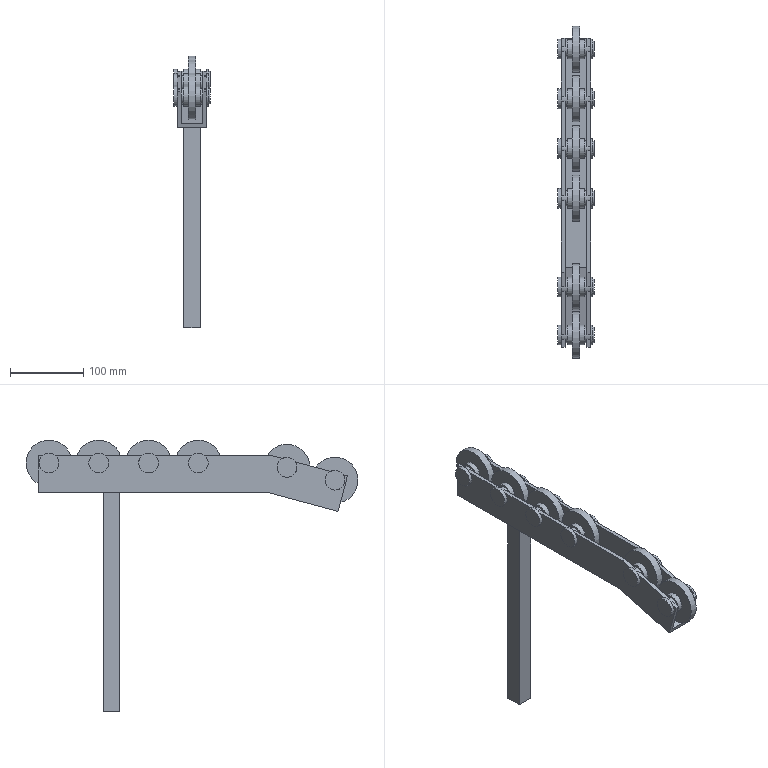Part | NX | features MAIN_BODY 2 | 1 solid | 138 faces | box 50 x 453.864 x 371.5 mm | volume 599471 mm3 | plane 90 | cylinder 48 | commonest cylinder face diameters 27 x24 21 x18 63 x6